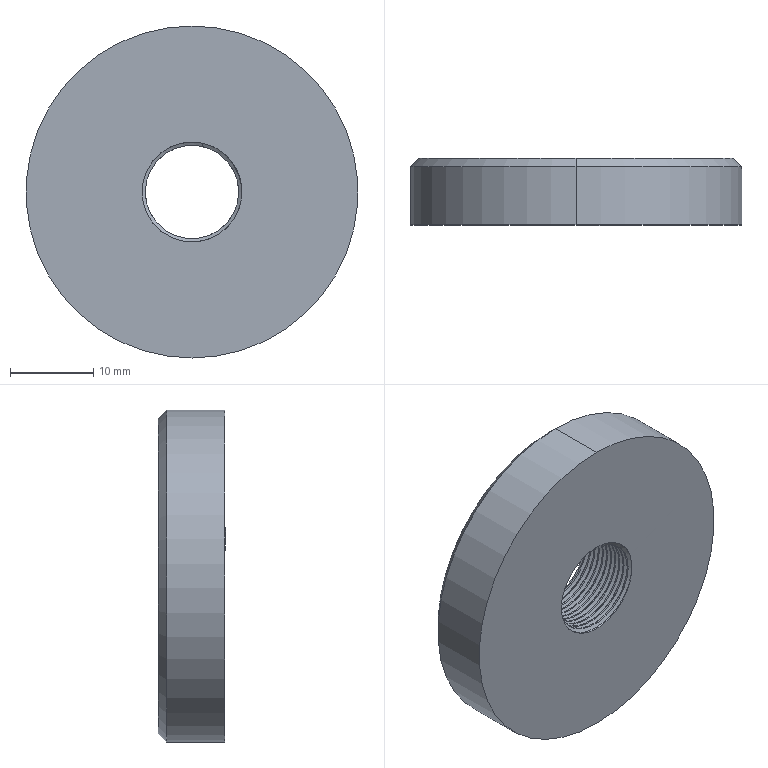Part | SolidWorks | features Chamfer 1, Extrusion 1, SweepThread 1 | 1 solid | 36 faces | box 39.9 x 8.112 x 39.9 mm | volume 9095 mm3 | cylinder 26 | plane 4 | spline 4 | cone 2 | commonest cylinder face diameters 12 x24 39.9 x2